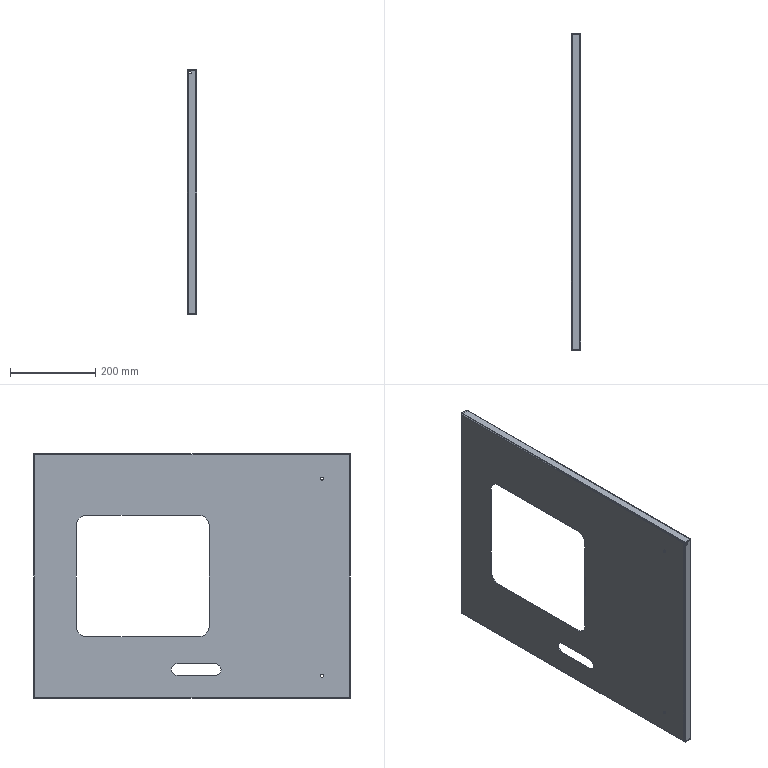Part | STEP file | Right Small Door | 1 solid | 115 faces | box 22 x 745 x 575 mm | volume 822578 mm3 | plane 68 | cylinder 31 | spline 16 | commonest cylinder face diameters 1 x8 5 x8 6 x4 7 x4 50 x4 27 x3